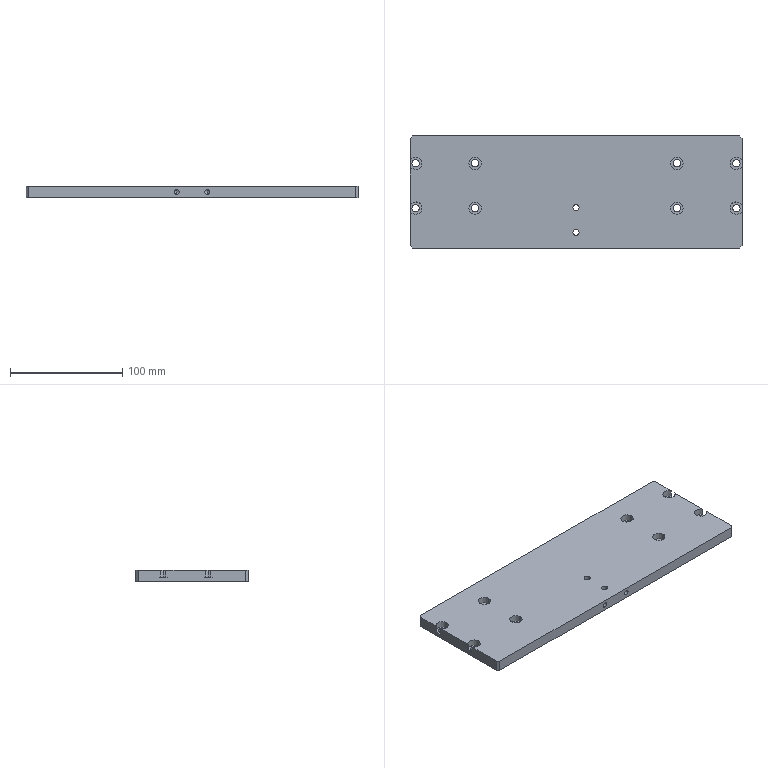Part | STEP file | mounting plate 6 | 1 solid | 66 faces | box 296 x 100 x 10 mm | volume 288795 mm3 | cylinder 42 | plane 20 | cone 4 | commonest cylinder face diameters 6.6 x16 11 x14 4.2 x4 5.5 x4 10 x4